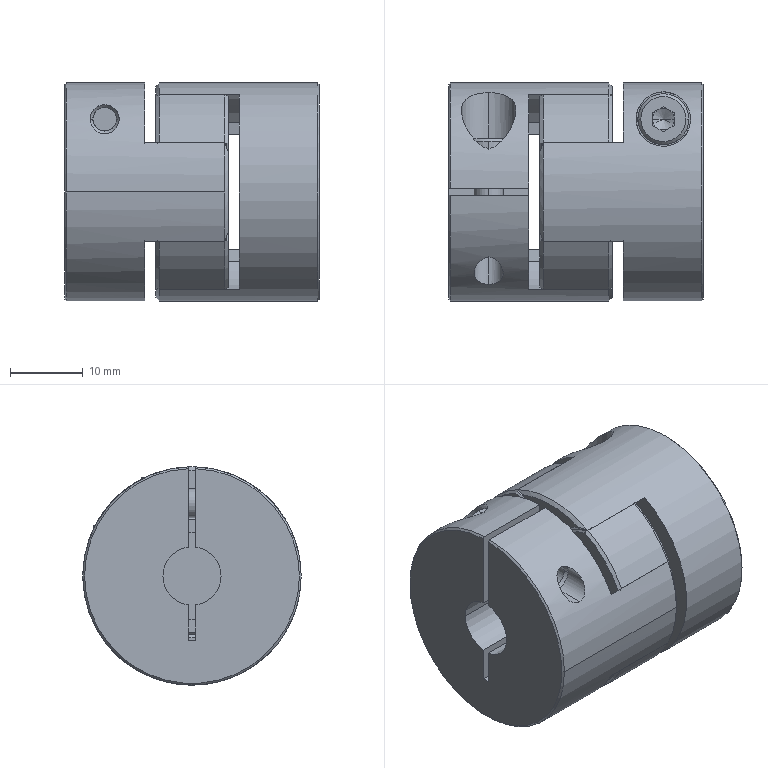Part | NX | 5 solids | 239 faces | box 35 x 30 x 30 mm | volume 20206 mm3 | plane 94 | cone 76 | cylinder 65 | torus 4 | commonest cylinder face diameters 16.982 x16 4 x12 16 x8 30 x8 3.242 x4 7 x4